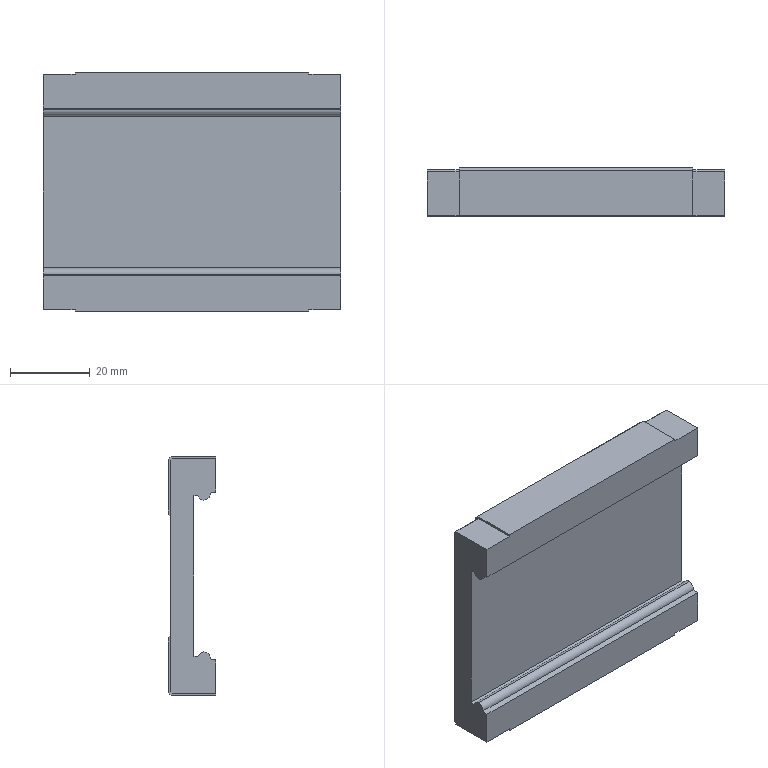Part | STEP file | Linear rail MR15WLSS1V1H-880L-20-20-I(S)_CPC_default | 1 solid | 61 faces | box 74.5 x 12 x 60 mm | volume 35281 mm3 | plane 34 | cylinder 19 | cone 8 | commonest cylinder face diameters 3.3 x8 4 x8 3.18 x3